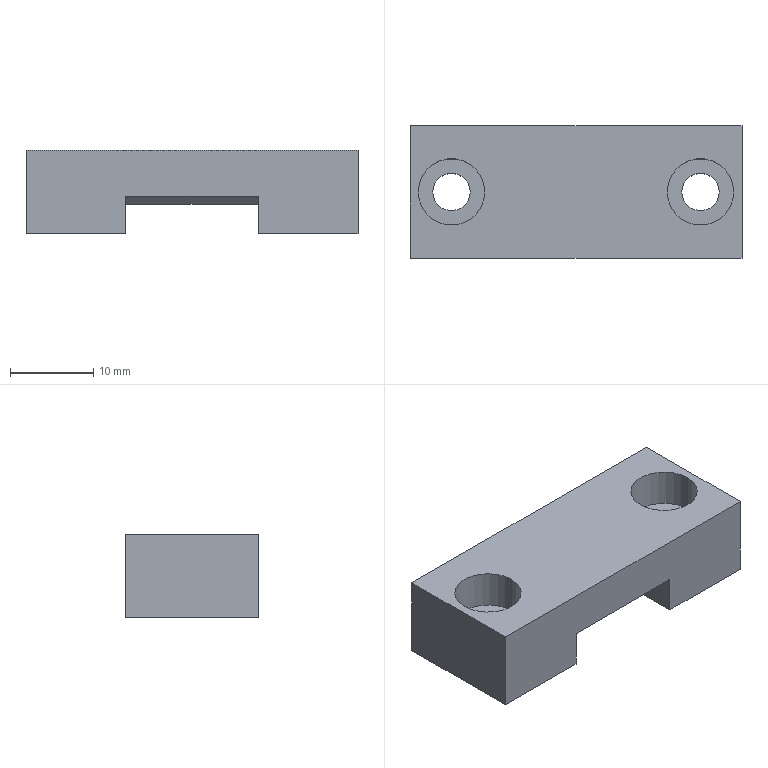Part | STEP file | PN_0023 Mount electronic clip pressure plate | 1 solid | 22 faces | box 40 x 16 x 10 mm | volume 4854 mm3 | plane 14 | cylinder 8 | commonest cylinder face diameters 4.5 x4 8 x4